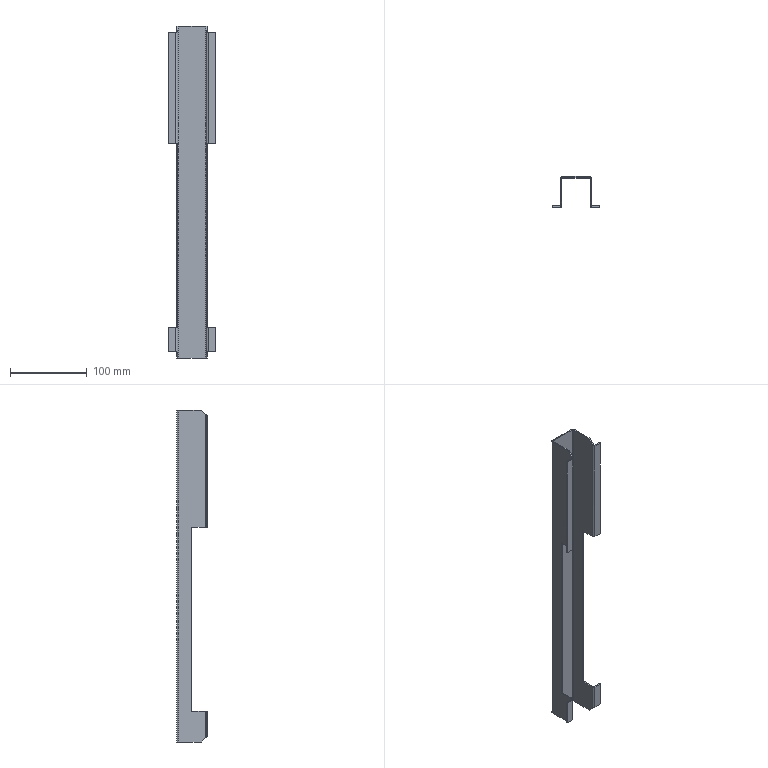Part | SolidWorks | features ICE 2, FlatPattern 1, SMBaseFlange 1, SheetMetal 1 | 1 solid | 58 faces | box 61 x 40 x 433 mm | volume 65237 mm3 | plane 42 | cylinder 12 | spline 4 | commonest cylinder face diameters 2 x6 5 x6